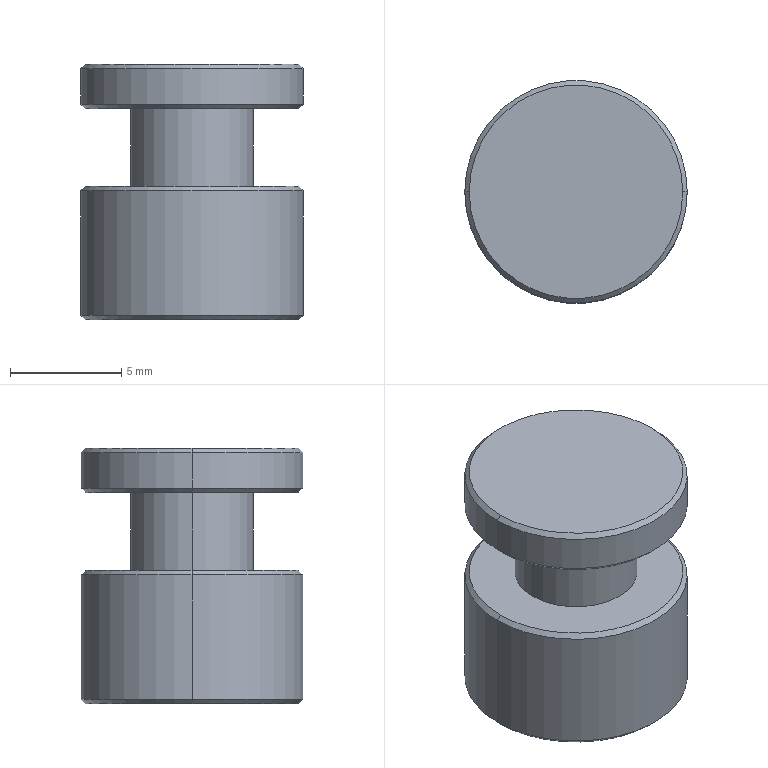Part | SolidWorks | features ICE 2, Chamfer 1, Extrusion 1, HoleWzd 1 | 1 solid | 22 faces | box 10 x 10 x 11.5 mm | volume 637.742 mm3 | cone 10 | cylinder 8 | plane 4 | commonest cylinder face diameters 10 x4 3.3 x2 5.5 x2
STEP:
#1=CARTESIAN_POINT('',(4.8,0.,11.5));
#2=VERTEX_POINT('',#1);
#3=CARTESIAN_POINT('',(-4.8,0.,11.5));
#4=VERTEX_POINT('',#3);
#5=CARTESIAN_POINT('',(0.,0.,11.5));
#6=DIRECTION('',(0.,0.,1.));
#7=DIRECTION('',(1.,0.,0.));
#8=AXIS2_PLACEMENT_3D('',#5,#6,#7);
#9=CIRCLE('',#8,4.8);
#10=EDGE_CURVE('',#2,#4,#9,.T.);
#11=ORIENTED_EDGE('',*,*,#10,.F.);
#12=CARTESIAN_POINT('',(5.,0.,11.3));
#13=VERTEX_POINT('',#12);
#14=CARTESIAN_POINT('',(4.8,0.,11.5));
#15=DIRECTION('',(0.7071,0.,-0.7071));
#16=VECTOR('',#15,1000.);
#17=LINE('',#14,#16);
#18=EDGE_CURVE('',#2,#13,#17,.T.);
#19=ORIENTED_EDGE('',*,*,#18,.T.);
#20=CARTESIAN_POINT('',(-5.,0.,11.3));
#21=VERTEX_POINT('',#20);
#22=CARTESIAN_POINT('',(0.,0.,11.3));
#23=DIRECTION('',(0.,0.,-1.));
#24=DIRECTION('',(1.,0.,0.));
#25=AXIS2_PLACEMENT_3D('',#22,#23,#24);
#26=CIRCLE('',#25,5.);
#27=EDGE_CURVE('',#21,#13,#26,.T.);
#28=ORIENTED_EDGE('',*,*,#27,.F.);
#29=CARTESIAN_POINT('',(-4.8,0.,11.5));
#30=DIRECTION('',(-0.7071,0.,-0.7071));
#31=VECTOR('',#30,1000.);
#32=LINE('',#29,#31);
#33=EDGE_CURVE('',#4,#21,#32,.T.);
#34=ORIENTED_EDGE('',*,*,#33,.F.);
#35=EDGE_LOOP('',(#11,#19,#28,#34));
#36=FACE_OUTER_BOUND('',#35,.T.);
#37=CARTESIAN_POINT('',(0.,0.,11.5));
#38=DIRECTION('',(0.,0.,-1.));
#39=DIRECTION('',(-1.,0.,0.));
#40=AXIS2_PLACEMENT_3D('',#37,#38,#39);
#41=CONICAL_SURFACE('',#40,4.8,0.7854);
#42=ADVANCED_FACE('',(#36),#41,.T.);
#43=CARTESIAN_POINT('',(-4.8,0.,9.5));
#44=VERTEX_POINT('',#43);
#45=CARTESIAN_POINT('',(4.8,0.,9.5));
#46=VERTEX_POINT('',#45);
#47=CARTESIAN_POINT('',(0.,0.,9.5));
#48=DIRECTION('',(0.,0.,-1.));
#49=DIRECTION('',(1.,0.,0.));
#50=AXIS2_PLACEMENT_3D('',#47,#48,#49);
#51=CIRCLE('',#50,4.8);
#52=EDGE_CURVE('',#44,#46,#51,.T.);
#53=ORIENTED_EDGE('',*,*,#52,.F.);
#54=CARTESIAN_POINT('',(-5.,0.,9.7));
#55=VERTEX_POINT('',#54);
#56=CARTESIAN_POINT('',(-5.,0.,9.7));
#57=DIRECTION('',(-0.7071,0.,0.7071));
#58=VECTOR('',#57,1000.);
#59=LINE('',#56,#58);
#60=EDGE_CURVE('',#44,#55,#59,.T.);
#61=ORIENTED_EDGE('',*,*,#60,.T.);
#62=CARTESIAN_POINT('',(5.,0.,9.7));
#63=VERTEX_POINT('',#62);
#64=CARTESIAN_POINT('',(0.,0.,9.7));
#65=DIRECTION('',(0.,0.,1.));
#66=DIRECTION('',(1.,0.,0.));
#67=AXIS2_PLACEMENT_3D('',#64,#65,#66);
#68=CIRCLE('',#67,5.);
#69=EDGE_CURVE('',#63,#55,#68,.T.);
#70=ORIENTED_EDGE('',*,*,#69,.F.);
#71=CARTESIAN_POINT('',(5.,0.,9.7));
#72=DIRECTION('',(0.7071,0.,0.7071));
#73=VECTOR('',#72,1000.);
#74=LINE('',#71,#73);
#75=EDGE_CURVE('',#46,#63,#74,.T.);
#76=ORIENTED_EDGE('',*,*,#75,.F.);
#77=EDGE_LOOP('',(#53,#61,#70,#76));
#78=FACE_OUTER_BOUND('',#77,.T.);
#79=CARTESIAN_POINT('',(0.,0.,9.7));
#80=DIRECTION('',(0.,0.,1.));
#81=DIRECTION('',(1.,0.,0.));
#82=AXIS2_PLACEMENT_3D('',#79,#80,#81);
#83=CONICAL_SURFACE('',#82,5.,0.7854);
#84=ADVANCED_FACE('',(#78),#83,.T.);
#85=CARTESIAN_POINT('',(4.8,0.,6.));
#86=VERTEX_POINT('',#85);
#87=CARTESIAN_POINT('',(-4.8,0.,6.));
#88=VERTEX_POINT('',#87);
#89=CARTESIAN_POINT('',(0.,0.,6.));
#90=DIRECTION('',(0.,0.,1.));
#91=DIRECTION('',(1.,0.,0.));
#92=AXIS2_PLACEMENT_3D('',#89,#90,#91);
#93=CIRCLE('',#92,4.8);
#94=EDGE_CURVE('',#86,#88,#93,.T.);
#95=ORIENTED_EDGE('',*,*,#94,.F.);
#96=CARTESIAN_POINT('',(5.,0.,5.8));
#97=VERTEX_POINT('',#96);
#98=CARTESIAN_POINT('',(4.8,0.,6.));
#99=DIRECTION('',(0.7071,0.,-0.7071));
#100=VECTOR('',#99,1000.);
#101=LINE('',#98,#100);
#102=EDGE_CURVE('',#86,#97,#101,.T.);
#103=ORIENTED_EDGE('',*,*,#102,.T.);
#104=CARTESIAN_POINT('',(-5.,0.,5.8));
#105=VERTEX_POINT('',#104);
#106=CARTESIAN_POINT('',(0.,0.,5.8));
#107=DIRECTION('',(0.,0.,-1.));
#108=DIRECTION('',(1.,0.,0.));
#109=AXIS2_PLACEMENT_3D('',#106,#107,#108);
#110=CIRCLE('',#109,5.);
#111=EDGE_CURVE('',#105,#97,#110,.T.);
#112=ORIENTED_EDGE('',*,*,#111,.F.);
#113=CARTESIAN_POINT('',(-4.8,0.,6.));
#114=DIRECTION('',(-0.7071,0.,-0.7071));
#115=VECTOR('',#114,1000.);
#116=LINE('',#113,#115);
#117=EDGE_CURVE('',#88,#105,#116,.T.);
#118=ORIENTED_EDGE('',*,*,#117,.F.);
#119=EDGE_LOOP('',(#95,#103,#112,#118));
#120=FACE_OUTER_BOUND('',#119,.T.);
#121=CARTESIAN_POINT('',(0.,0.,6.));
#122=DIRECTION('',(0.,0.,-1.));
#123=DIRECTION('',(-1.,0.,0.));
#124=AXIS2_PLACEMENT_3D('',#121,#122,#123);
#125=CONICAL_SURFACE('',#124,4.8,0.7854);
#126=ADVANCED_FACE('',(#120),#125,.T.);
#127=CARTESIAN_POINT('',(-4.8,0.,0.));
#128=VERTEX_POINT('',#127);
#129=CARTESIAN_POINT('',(4.8,0.,0.));
#130=VERTEX_POINT('',#129);
#131=CARTESIAN_POINT('',(0.,0.,0.));
#132=DIRECTION('',(0.,0.,-1.));
#133=DIRECTION('',(1.,0.,0.));
#134=AXIS2_PLACEMENT_3D('',#131,#132,#133);
#135=CIRCLE('',#134,4.8);
#136=EDGE_CURVE('',#128,#130,#135,.T.);
#137=ORIENTED_EDGE('',*,*,#136,.F.);
#138=CARTESIAN_POINT('',(-5.,0.,0.2));
#139=VERTEX_POINT('',#138);
#140=CARTESIAN_POINT('',(-5.,0.,0.2));
#141=DIRECTION('',(-0.7071,0.,0.7071));
#142=VECTOR('',#141,1000.);
#143=LINE('',#140,#142);
#144=EDGE_CURVE('',#128,#139,#143,.T.);
#145=ORIENTED_EDGE('',*,*,#144,.T.);
#146=CARTESIAN_POINT('',(5.,0.,0.2));
#147=VERTEX_POINT('',#146);
#148=CARTESIAN_POINT('',(0.,0.,0.2));
#149=DIRECTION('',(0.,0.,1.));
#150=DIRECTION('',(1.,0.,0.));
#151=AXIS2_PLACEMENT_3D('',#148,#149,#150);
#152=CIRCLE('',#151,5.);
#153=EDGE_CURVE('',#147,#139,#152,.T.);
#154=ORIENTED_EDGE('',*,*,#153,.F.);
#155=CARTESIAN_POINT('',(5.,0.,0.2));
#156=DIRECTION('',(0.7071,0.,0.7071));
#157=VECTOR('',#156,1000.);
#158=LINE('',#155,#157);
#159=EDGE_CURVE('',#130,#147,#158,.T.);
#160=ORIENTED_EDGE('',*,*,#159,.F.);
#161=EDGE_LOOP('',(#137,#145,#154,#160));
#162=FACE_OUTER_BOUND('',#161,.T.);
#163=CARTESIAN_POINT('',(0.,0.,0.2));
#164=DIRECTION('',(0.,0.,1.));
#165=DIRECTION('',(1.,0.,0.));
#166=AXIS2_PLACEMENT_3D('',#163,#164,#165);
#167=CONICAL_SURFACE('',#166,5.,0.7854);
#168=ADVANCED_FACE('',(#162),#167,.T.);
#169=CARTESIAN_POINT('',(1.65,0.,8.));
#170=VERTEX_POINT('',#169);
#171=CARTESIAN_POINT('',(-1.65,0.,8.));
#172=VERTEX_POINT('',#171);
#173=CARTESIAN_POINT('',(0.,0.,8.));
#174=DIRECTION('',(0.,0.,-1.));
#175=DIRECTION('',(-1.,0.,0.));
#176=AXIS2_PLACEMENT_3D('',#173,#174,#175);
#177=CIRCLE('',#176,1.65);
#178=EDGE_CURVE('',#170,#172,#177,.T.);
#179=ORIENTED_EDGE('',*,*,#178,.F.);
#180=CARTESIAN_POINT('',(1.65,0.,0.));
#181=VERTEX_POINT('',#180);
#182=CARTESIAN_POINT('',(1.65,0.,0.));
#183=DIRECTION('',(0.,0.,-1.));
#184=VECTOR('',#183,1000.);
#185=LINE('',#182,#184);
#186=EDGE_CURVE('',#170,#181,#185,.T.);
#187=ORIENTED_EDGE('',*,*,#186,.T.);
#188=CARTESIAN_POINT('',(-1.65,0.,0.));
#189=VERTEX_POINT('',#188);
#190=CARTESIAN_POINT('',(0.,0.,0.));
#191=DIRECTION('',(0.,0.,-1.));
#192=DIRECTION('',(-1.,0.,0.));
#193=AXIS2_PLACEMENT_3D('',#190,#191,#192);
#194=CIRCLE('',#193,1.65);
#195=EDGE_CURVE('',#181,#189,#194,.T.);
#196=ORIENTED_EDGE('',*,*,#195,.T.);
#197=CARTESIAN_POINT('',(-1.65,0.,0.));
#198=DIRECTION('',(0.,0.,-1.));
#199=VECTOR('',#198,1000.);
#200=LINE('',#197,#199);
#201=EDGE_CURVE('',#172,#189,#200,.T.);
#202=ORIENTED_EDGE('',*,*,#201,.F.);
#203=EDGE_LOOP('',(#179,#187,#196,#202));
#204=FACE_OUTER_BOUND('',#203,.T.);
#205=CARTESIAN_POINT('',(0.,0.,0.));
#206=DIRECTION('',(0.,0.,-1.));
#207=DIRECTION('',(-1.,0.,0.));
#208=AXIS2_PLACEMENT_3D('',#205,#206,#207);
#209=CYLINDRICAL_SURFACE('',#208,1.65);
#210=ADVANCED_FACE('',(#204),#209,.F.);
#211=CARTESIAN_POINT('',(0.,0.,8.991));
#212=VERTEX_POINT('',#211);
#213=CARTESIAN_POINT('',(-1.65,0.,8.));
#214=DIRECTION('',(-0.8572,0.,-0.515));
#215=VECTOR('',#214,1000.);
#216=LINE('',#213,#215);
#217=EDGE_CURVE('',#212,#172,#216,.T.);
#218=ORIENTED_EDGE('',*,*,#217,.F.);
#219=CARTESIAN_POINT('',(1.65,0.,8.));
#220=DIRECTION('',(0.8572,0.,-0.515));
#221=VECTOR('',#220,1000.);
#222=LINE('',#219,#221);
#223=EDGE_CURVE('',#212,#170,#222,.T.);
#224=ORIENTED_EDGE('',*,*,#223,.T.);
#225=ORIENTED_EDGE('',*,*,#178,.T.);
#226=EDGE_LOOP('',(#218,#224,#225));
#227=FACE_OUTER_BOUND('',#226,.T.);
#228=CARTESIAN_POINT('',(0.,0.,8.));
#229=DIRECTION('',(0.,0.,-1.));
#230=DIRECTION('',(-1.,0.,0.));
#231=AXIS2_PLACEMENT_3D('',#228,#229,#230);
#232=CONICAL_SURFACE('',#231,1.65,1.03);
#233=ADVANCED_FACE('',(#227),#232,.F.);
#234=ORIENTED_EDGE('',*,*,#27,.T.);
#235=CARTESIAN_POINT('',(5.,0.,11.5));
#236=DIRECTION('',(0.,0.,-1.));
#237=VECTOR('',#236,1000.);
#238=LINE('',#235,#237);
#239=EDGE_CURVE('',#13,#63,#238,.T.);
#240=ORIENTED_EDGE('',*,*,#239,.T.);
#241=ORIENTED_EDGE('',*,*,#69,.T.);
#242=CARTESIAN_POINT('',(-5.,0.,11.5));
#243=DIRECTION('',(0.,0.,-1.));
#244=VECTOR('',#243,1000.);
#245=LINE('',#242,#244);
#246=EDGE_CURVE('',#21,#55,#245,.T.);
#247=ORIENTED_EDGE('',*,*,#246,.F.);
#248=EDGE_LOOP('',(#234,#240,#241,#247));
#249=FACE_OUTER_BOUND('',#248,.T.);
#250=CARTESIAN_POINT('',(0.,0.,11.5));
#251=DIRECTION('',(0.,0.,-1.));
#252=DIRECTION('',(-1.,0.,0.));
#253=AXIS2_PLACEMENT_3D('',#250,#251,#252);
#254=CYLINDRICAL_SURFACE('',#253,5.);
#255=ADVANCED_FACE('',(#249),#254,.T.);
#256=CARTESIAN_POINT('',(2.75,0.,9.5));
#257=VERTEX_POINT('',#256);
#258=CARTESIAN_POINT('',(-2.75,0.,9.5));
#259=VERTEX_POINT('',#258);
#260=CARTESIAN_POINT('',(0.,0.,9.5));
#261=DIRECTION('',(0.,0.,1.));
#262=DIRECTION('',(1.,0.,0.));
#263=AXIS2_PLACEMENT_3D('',#260,#261,#262);
#264=CIRCLE('',#263,2.75);
#265=EDGE_CURVE('',#257,#259,#264,.T.);
#266=ORIENTED_EDGE('',*,*,#265,.F.);
#267=CARTESIAN_POINT('',(2.75,0.,6.));
#268=VERTEX_POINT('',#267);
#269=CARTESIAN_POINT('',(2.75,0.,9.5));
#270=DIRECTION('',(0.,0.,-1.));
#271=VECTOR('',#270,1000.);
#272=LINE('',#269,#271);
#273=EDGE_CURVE('',#257,#268,#272,.T.);
#274=ORIENTED_EDGE('',*,*,#273,.T.);
#275=CARTESIAN_POINT('',(-2.75,0.,6.));
#276=VERTEX_POINT('',#275);
#277=CARTESIAN_POINT('',(0.,0.,6.));
#278=DIRECTION('',(0.,0.,1.));
#279=DIRECTION('',(1.,0.,0.));
#280=AXIS2_PLACEMENT_3D('',#277,#278,#279);
#281=CIRCLE('',#280,2.75);
#282=EDGE_CURVE('',#268,#276,#281,.T.);
#283=ORIENTED_EDGE('',*,*,#282,.T.);
#284=CARTESIAN_POINT('',(-2.75,0.,9.5));
#285=DIRECTION('',(0.,0.,-1.));
#286=VECTOR('',#285,1000.);
#287=LINE('',#284,#286);
#288=EDGE_CURVE('',#259,#276,#287,.T.);
#289=ORIENTED_EDGE('',*,*,#288,.F.);
#290=EDGE_LOOP('',(#266,#274,#283,#289));
#291=FACE_OUTER_BOUND('',#290,.T.);
#292=CARTESIAN_POINT('',(0.,0.,9.5));
#293=DIRECTION('',(0.,0.,-1.));
#294=DIRECTION('',(-1.,0.,0.));
#295=AXIS2_PLACEMENT_3D('',#292,#293,#294);
#296=CYLINDRICAL_SURFACE('',#295,2.75);
#297=ADVANCED_FACE('',(#291),#296,.T.);
#298=ORIENTED_EDGE('',*,*,#111,.T.);
#299=CARTESIAN_POINT('',(5.,0.,6.));
#300=DIRECTION('',(0.,0.,-1.));
#301=VECTOR('',#300,1000.);
#302=LINE('',#299,#301);
#303=EDGE_CURVE('',#97,#147,#302,.T.);
#304=ORIENTED_EDGE('',*,*,#303,.T.);
#305=ORIENTED_EDGE('',*,*,#153,.T.);
#306=CARTESIAN_POINT('',(-5.,0.,6.));
#307=DIRECTION('',(0.,0.,-1.));
#308=VECTOR('',#307,1000.);
#309=LINE('',#306,#308);
#310=EDGE_CURVE('',#105,#139,#309,.T.);
#311=ORIENTED_EDGE('',*,*,#310,.F.);
#312=EDGE_LOOP('',(#298,#304,#305,#311));
#313=FACE_OUTER_BOUND('',#312,.T.);
#314=CARTESIAN_POINT('',(0.,0.,6.));
#315=DIRECTION('',(0.,0.,-1.));
#316=DIRECTION('',(-1.,0.,0.));
#317=AXIS2_PLACEMENT_3D('',#314,#315,#316);
#318=CYLINDRICAL_SURFACE('',#317,5.);
#319=ADVANCED_FACE('',(#313),#318,.T.);
#320=CARTESIAN_POINT('',(0.,0.,6.));
#321=DIRECTION('',(0.,0.,1.));
#322=DIRECTION('',(1.,0.,0.));
#323=AXIS2_PLACEMENT_3D('',#320,#321,#322);
#324=CIRCLE('',#323,4.8);
#325=EDGE_CURVE('',#88,#86,#324,.T.);
#326=ORIENTED_EDGE('',*,*,#325,.T.);
#327=ORIENTED_EDGE('',*,*,#94,.T.);
#328=EDGE_LOOP('',(#326,#327));
#329=FACE_OUTER_BOUND('',#328,.T.);
#330=CARTESIAN_POINT('',(0.,0.,6.));
#331=DIRECTION('',(0.,0.,1.));
#332=DIRECTION('',(1.,0.,0.));
#333=AXIS2_PLACEMENT_3D('',#330,#331,#332);
#334=CIRCLE('',#333,2.75);
#335=EDGE_CURVE('',#276,#268,#334,.T.);
#336=ORIENTED_EDGE('',*,*,#335,.F.);
#337=ORIENTED_EDGE('',*,*,#282,.F.);
#338=EDGE_LOOP('',(#336,#337));
#339=FACE_BOUND('',#338,.T.);
#340=CARTESIAN_POINT('',(0.,0.,6.));
#341=DIRECTION('',(0.,0.,1.));
#342=DIRECTION('',(1.,0.,0.));
#343=AXIS2_PLACEMENT_3D('',#340,#341,#342);
#344=PLANE('',#343);
#345=ADVANCED_FACE('',(#329,#339),#344,.T.);
#346=ORIENTED_EDGE('',*,*,#303,.F.);
#347=CARTESIAN_POINT('',(0.,0.,5.8));
#348=DIRECTION('',(0.,0.,-1.));
#349=DIRECTION('',(1.,0.,0.));
#350=AXIS2_PLACEMENT_3D('',#347,#348,#349);
#351=CIRCLE('',#350,5.);
#352=EDGE_CURVE('',#97,#105,#351,.T.);
#353=ORIENTED_EDGE('',*,*,#352,.T.);
#354=ORIENTED_EDGE('',*,*,#310,.T.);
#355=CARTESIAN_POINT('',(0.,0.,0.2));
#356=DIRECTION('',(0.,0.,1.));
#357=DIRECTION('',(1.,0.,0.));
#358=AXIS2_PLACEMENT_3D('',#355,#356,#357);
#359=CIRCLE('',#358,5.);
#360=EDGE_CURVE('',#139,#147,#359,.T.);
#361=ORIENTED_EDGE('',*,*,#360,.T.);
#362=EDGE_LOOP('',(#346,#353,#354,#361));
#363=FACE_OUTER_BOUND('',#362,.T.);
#364=CARTESIAN_POINT('',(0.,0.,6.));
#365=DIRECTION('',(0.,0.,-1.));
#366=DIRECTION('',(-1.,0.,0.));
#367=AXIS2_PLACEMENT_3D('',#364,#365,#366);
#368=CYLINDRICAL_SURFACE('',#367,5.);
#369=ADVANCED_FACE('',(#363),#368,.T.);
#370=CARTESIAN_POINT('',(0.,0.,0.));
#371=DIRECTION('',(0.,0.,-1.));
#372=DIRECTION('',(1.,0.,0.));
#373=AXIS2_PLACEMENT_3D('',#370,#371,#372);
#374=CIRCLE('',#373,4.8);
#375=EDGE_CURVE('',#130,#128,#374,.T.);
#376=ORIENTED_EDGE('',*,*,#375,.T.);
#377=ORIENTED_EDGE('',*,*,#136,.T.);
#378=EDGE_LOOP('',(#376,#377));
#379=FACE_OUTER_BOUND('',#378,.T.);
#380=CARTESIAN_POINT('',(0.,0.,0.));
#381=DIRECTION('',(0.,0.,-1.));
#382=DIRECTION('',(-1.,0.,0.));
#383=AXIS2_PLACEMENT_3D('',#380,#381,#382);
#384=CIRCLE('',#383,1.65);
#385=EDGE_CURVE('',#189,#181,#384,.T.);
#386=ORIENTED_EDGE('',*,*,#385,.F.);
#387=ORIENTED_EDGE('',*,*,#195,.F.);
#388=EDGE_LOOP('',(#386,#387));
#389=FACE_BOUND('',#388,.T.);
#390=CARTESIAN_POINT('',(0.,0.,0.));
#391=DIRECTION('',(0.,0.,1.));
#392=DIRECTION('',(1.,0.,0.));
#393=AXIS2_PLACEMENT_3D('',#390,#391,#392);
#394=PLANE('',#393);
#395=ADVANCED_FACE('',(#379,#389),#394,.F.);
#396=ORIENTED_EDGE('',*,*,#273,.F.);
#397=CARTESIAN_POINT('',(0.,0.,9.5));
#398=DIRECTION('',(0.,0.,1.));
#399=DIRECTION('',(1.,0.,0.));
#400=AXIS2_PLACEMENT_3D('',#397,#398,#399);
#401=CIRCLE('',#400,2.75);
#402=EDGE_CURVE('',#259,#257,#401,.T.);
#403=ORIENTED_EDGE('',*,*,#402,.F.);
#404=ORIENTED_EDGE('',*,*,#288,.T.);
#405=ORIENTED_EDGE('',*,*,#335,.T.);
#406=EDGE_LOOP('',(#396,#403,#404,#405));
#407=FACE_OUTER_BOUND('',#406,.T.);
#408=CARTESIAN_POINT('',(0.,0.,9.5));
#409=DIRECTION('',(0.,0.,-1.));
#410=DIRECTION('',(-1.,0.,0.));
#411=AXIS2_PLACEMENT_3D('',#408,#409,#410);
#412=CYLINDRICAL_SURFACE('',#411,2.75);
#413=ADVANCED_FACE('',(#407),#412,.T.);
#414=CARTESIAN_POINT('',(0.,0.,9.5));
#415=DIRECTION('',(0.,0.,-1.));
#416=DIRECTION('',(1.,0.,0.));
#417=AXIS2_PLACEMENT_3D('',#414,#415,#416);
#418=CIRCLE('',#417,4.8);
#419=EDGE_CURVE('',#46,#44,#418,.T.);
#420=ORIENTED_EDGE('',*,*,#419,.T.);
#421=ORIENTED_EDGE('',*,*,#52,.T.);
#422=EDGE_LOOP('',(#420,#421));
#423=FACE_OUTER_BOUND('',#422,.T.);
#424=ORIENTED_EDGE('',*,*,#402,.T.);
#425=ORIENTED_EDGE('',*,*,#265,.T.);
#426=EDGE_LOOP('',(#424,#425));
#427=FACE_BOUND('',#426,.T.);
#428=CARTESIAN_POINT('',(0.,0.,9.5));
#429=DIRECTION('',(0.,0.,1.));
#430=DIRECTION('',(1.,0.,0.));
#431=AXIS2_PLACEMENT_3D('',#428,#429,#430);
#432=PLANE('',#431);
#433=ADVANCED_FACE('',(#423,#427),#432,.F.);
#434=ORIENTED_EDGE('',*,*,#239,.F.);
#435=CARTESIAN_POINT('',(0.,0.,11.3));
#436=DIRECTION('',(0.,0.,-1.));
#437=DIRECTION('',(1.,0.,0.));
#438=AXIS2_PLACEMENT_3D('',#435,#436,#437);
#439=CIRCLE('',#438,5.);
#440=EDGE_CURVE('',#13,#21,#439,.T.);
#441=ORIENTED_EDGE('',*,*,#440,.T.);
#442=ORIENTED_EDGE('',*,*,#246,.T.);
#443=CARTESIAN_POINT('',(0.,0.,9.7));
#444=DIRECTION('',(0.,0.,1.));
#445=DIRECTION('',(1.,0.,0.));
#446=AXIS2_PLACEMENT_3D('',#443,#444,#445);
#447=CIRCLE('',#446,5.);
#448=EDGE_CURVE('',#55,#63,#447,.T.);
#449=ORIENTED_EDGE('',*,*,#448,.T.);
#450=EDGE_LOOP('',(#434,#441,#442,#449));
#451=FACE_OUTER_BOUND('',#450,.T.);
#452=CARTESIAN_POINT('',(0.,0.,11.5));
#453=DIRECTION('',(0.,0.,-1.));
#454=DIRECTION('',(-1.,0.,0.));
#455=AXIS2_PLACEMENT_3D('',#452,#453,#454);
#456=CYLINDRICAL_SURFACE('',#455,5.);
#457=ADVANCED_FACE('',(#451),#456,.T.);
#458=CARTESIAN_POINT('',(0.,0.,11.5));
#459=DIRECTION('',(0.,0.,1.));
#460=DIRECTION('',(1.,0.,0.));
#461=AXIS2_PLACEMENT_3D('',#458,#459,#460);
#462=CIRCLE('',#461,4.8);
#463=EDGE_CURVE('',#4,#2,#462,.T.);
#464=ORIENTED_EDGE('',*,*,#463,.T.);
#465=ORIENTED_EDGE('',*,*,#10,.T.);
#466=EDGE_LOOP('',(#464,#465));
#467=FACE_OUTER_BOUND('',#466,.T.);
#468=CARTESIAN_POINT('',(0.,0.,11.5));
#469=DIRECTION('',(0.,0.,1.));
#470=DIRECTION('',(1.,0.,0.));
#471=AXIS2_PLACEMENT_3D('',#468,#469,#470);
#472=PLANE('',#471);
#473=ADVANCED_FACE('',(#467),#472,.T.);
#474=ORIENTED_EDGE('',*,*,#223,.F.);
#475=ORIENTED_EDGE('',*,*,#217,.T.);
#476=CARTESIAN_POINT('',(0.,0.,8.));
#477=DIRECTION('',(0.,0.,-1.));
#478=DIRECTION('',(-1.,0.,0.));
#479=AXIS2_PLACEMENT_3D('',#476,#477,#478);
#480=CIRCLE('',#479,1.65);
#481=EDGE_CURVE('',#172,#170,#480,.T.);
#482=ORIENTED_EDGE('',*,*,#481,.T.);
#483=EDGE_LOOP('',(#474,#475,#482));
#484=FACE_OUTER_BOUND('',#483,.T.);
#485=CARTESIAN_POINT('',(0.,0.,8.));
#486=DIRECTION('',(0.,0.,-1.));
#487=DIRECTION('',(-1.,0.,0.));
#488=AXIS2_PLACEMENT_3D('',#485,#486,#487);
#489=CONICAL_SURFACE('',#488,1.65,1.03);
#490=ADVANCED_FACE('',(#484),#489,.F.);
#491=ORIENTED_EDGE('',*,*,#186,.F.);
#492=ORIENTED_EDGE('',*,*,#481,.F.);
#493=ORIENTED_EDGE('',*,*,#201,.T.);
#494=ORIENTED_EDGE('',*,*,#385,.T.);
#495=EDGE_LOOP('',(#491,#492,#493,#494));
#496=FACE_OUTER_BOUND('',#495,.T.);
#497=CARTESIAN_POINT('',(0.,0.,0.));
#498=DIRECTION('',(0.,0.,-1.));
#499=DIRECTION('',(-1.,0.,0.));
#500=AXIS2_PLACEMENT_3D('',#497,#498,#499);
#501=CYLINDRICAL_SURFACE('',#500,1.65);
#502=ADVANCED_FACE('',(#496),#501,.F.);
#503=ORIENTED_EDGE('',*,*,#144,.F.);
#504=ORIENTED_EDGE('',*,*,#375,.F.);
#505=ORIENTED_EDGE('',*,*,#159,.T.);
#506=ORIENTED_EDGE('',*,*,#360,.F.);
#507=EDGE_LOOP('',(#503,#504,#505,#506));
#508=FACE_OUTER_BOUND('',#507,.T.);
#509=CARTESIAN_POINT('',(0.,0.,0.2));
#510=DIRECTION('',(0.,0.,1.));
#511=DIRECTION('',(1.,0.,0.));
#512=AXIS2_PLACEMENT_3D('',#509,#510,#511);
#513=CONICAL_SURFACE('',#512,5.,0.7854);
#514=ADVANCED_FACE('',(#508),#513,.T.);
#515=ORIENTED_EDGE('',*,*,#102,.F.);
#516=ORIENTED_EDGE('',*,*,#325,.F.);
#517=ORIENTED_EDGE('',*,*,#117,.T.);
#518=ORIENTED_EDGE('',*,*,#352,.F.);
#519=EDGE_LOOP('',(#515,#516,#517,#518));
#520=FACE_OUTER_BOUND('',#519,.T.);
#521=CARTESIAN_POINT('',(0.,0.,6.));
#522=DIRECTION('',(0.,0.,-1.));
#523=DIRECTION('',(-1.,0.,0.));
#524=AXIS2_PLACEMENT_3D('',#521,#522,#523);
#525=CONICAL_SURFACE('',#524,4.8,0.7854);
#526=ADVANCED_FACE('',(#520),#525,.T.);
#527=ORIENTED_EDGE('',*,*,#60,.F.);
#528=ORIENTED_EDGE('',*,*,#419,.F.);
#529=ORIENTED_EDGE('',*,*,#75,.T.);
#530=ORIENTED_EDGE('',*,*,#448,.F.);
#531=EDGE_LOOP('',(#527,#528,#529,#530));
#532=FACE_OUTER_BOUND('',#531,.T.);
#533=CARTESIAN_POINT('',(0.,0.,9.7));
#534=DIRECTION('',(0.,0.,1.));
#535=DIRECTION('',(1.,0.,0.));
#536=AXIS2_PLACEMENT_3D('',#533,#534,#535);
#537=CONICAL_SURFACE('',#536,5.,0.7854);
#538=ADVANCED_FACE('',(#532),#537,.T.);
#539=ORIENTED_EDGE('',*,*,#18,.F.);
#540=ORIENTED_EDGE('',*,*,#463,.F.);
#541=ORIENTED_EDGE('',*,*,#33,.T.);
#542=ORIENTED_EDGE('',*,*,#440,.F.);
#543=EDGE_LOOP('',(#539,#540,#541,#542));
#544=FACE_OUTER_BOUND('',#543,.T.);
#545=CARTESIAN_POINT('',(0.,0.,11.5));
#546=DIRECTION('',(0.,0.,-1.));
#547=DIRECTION('',(-1.,0.,0.));
#548=AXIS2_PLACEMENT_3D('',#545,#546,#547);
#549=CONICAL_SURFACE('',#548,4.8,0.7854);
#550=ADVANCED_FACE('',(#544),#549,.T.);
#551=CLOSED_SHELL('',(#42,#84,#126,#168,#210,#233,#255,#297,#319,#345,#369,#395,#413,#433,#457,#473,#490,#502,#514,#526,#538,#550));
#552=MANIFOLD_SOLID_BREP('',#551);
#553=CARTESIAN_POINT('',(0.,0.,0.));
#554=DIRECTION('',(0.,0.,1.));
#555=DIRECTION('',(1.,0.,0.));
#556=AXIS2_PLACEMENT_3D('',#553,#554,#555);
#557=(LENGTH_UNIT()NAMED_UNIT(*)SI_UNIT(.MILLI.,.METRE.));
#558=UNCERTAINTY_MEASURE_WITH_UNIT(LENGTH_MEASURE(0.00001),#557,'','');
#559=(NAMED_UNIT(*)PLANE_ANGLE_UNIT()SI_UNIT($,.RADIAN.));
#560=(NAMED_UNIT(*)SI_UNIT($,.STERADIAN.)SOLID_ANGLE_UNIT());
#561=(GEOMETRIC_REPRESENTATION_CONTEXT(3)GLOBAL_UNCERTAINTY_ASSIGNED_CONTEXT((#558))GLOBAL_UNIT_ASSIGNED_CONTEXT((#557,#559,#560))REPRESENTATION_CONTEXT('',''));
#562=ADVANCED_BREP_SHAPE_REPRESENTATION('',(#552,#556),#561);